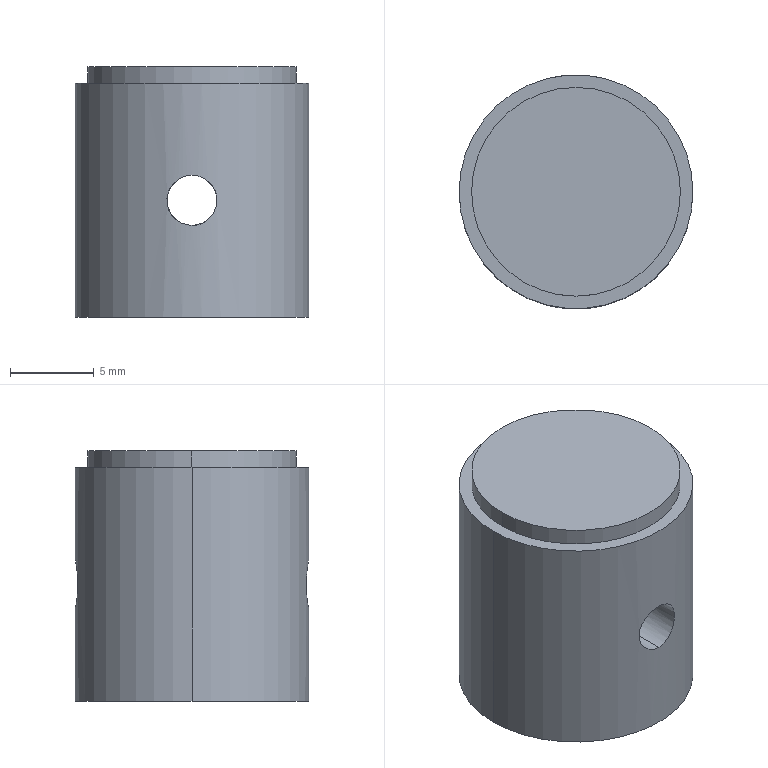Part | SolidWorks | features ICE 3, 3DProfileFeature 1, Extrusion 1, HoleWzd 1 | 1 solid | 17 faces | box 14 x 14 x 15 mm | volume 1304 mm3 | cylinder 10 | cone 4 | plane 3 | commonest cylinder face diameters 3 x4 9.5 x2 12.5 x2 14 x2
STEP:
#1=CARTESIAN_POINT('',(0.,-7.,5.5));
#2=VERTEX_POINT('',#1);
#3=CARTESIAN_POINT('',(0.,-7.,8.5));
#4=VERTEX_POINT('',#3);
#5=CARTESIAN_POINT('',(0.,-7.,5.5));
#6=CARTESIAN_POINT('',(-0.1961,-7.,5.5));
#7=CARTESIAN_POINT('',(-0.394,-6.991,5.54));
#8=CARTESIAN_POINT('',(-0.7552,-6.962,5.689));
#9=CARTESIAN_POINT('',(-0.9218,-6.94,5.801));
#10=CARTESIAN_POINT('',(-1.129,-6.909,6.008));
#11=CARTESIAN_POINT('',(-1.192,-6.898,6.085));
#12=CARTESIAN_POINT('',(-1.301,-6.878,6.247));
#13=CARTESIAN_POINT('',(-1.347,-6.869,6.333));
#14=CARTESIAN_POINT('',(-1.461,-6.846,6.606));
#15=CARTESIAN_POINT('',(-1.5,-6.837,6.801));
#16=CARTESIAN_POINT('',(-1.5,-6.837,7.098));
#17=CARTESIAN_POINT('',(-1.49,-6.84,7.196));
#18=CARTESIAN_POINT('',(-1.452,-6.848,7.388));
#19=CARTESIAN_POINT('',(-1.423,-6.854,7.484));
#20=CARTESIAN_POINT('',(-1.311,-6.877,7.756));
#21=CARTESIAN_POINT('',(-1.199,-6.898,7.922));
#22=CARTESIAN_POINT('',(-0.9236,-6.94,8.198));
#23=CARTESIAN_POINT('',(-0.7569,-6.961,8.31));
#24=CARTESIAN_POINT('',(-0.396,-6.991,8.46));
#25=CARTESIAN_POINT('',(-0.1988,-7.,8.5));
#26=CARTESIAN_POINT('',(0.,-7.,8.5));
#27=B_SPLINE_CURVE_WITH_KNOTS('',3,(#5,#6,#7,#8,#9,#10,#11,#12,#13,#14,#15,#16,#17,#18,#19,#20,#21,#22,#23,#24,#25,#26),.UNSPECIFIED.,.F.,.F.,(4,2,2,2,2,2,2,2,2,2,4),(0.004703,0.005291,0.005879,0.006173,0.006467,0.007054,0.007348,0.007642,0.00823,0.008818,0.009405),.UNSPECIFIED.);
#28=EDGE_CURVE('',#2,#4,#27,.T.);
#29=ORIENTED_EDGE('',*,*,#28,.F.);
#30=CARTESIAN_POINT('',(0.,-4.75,5.5));
#31=VERTEX_POINT('',#30);
#32=CARTESIAN_POINT('',(0.,-10.,5.5));
#33=DIRECTION('',(0.,1.,0.));
#34=VECTOR('',#33,1000.);
#35=LINE('',#32,#34);
#36=EDGE_CURVE('',#2,#31,#35,.T.);
#37=ORIENTED_EDGE('',*,*,#36,.T.);
#38=CARTESIAN_POINT('',(0.,-4.75,8.5));
#39=VERTEX_POINT('',#38);
#40=CARTESIAN_POINT('',(0.,-4.75,8.5));
#41=CARTESIAN_POINT('',(-0.0998,-4.75,8.5));
#42=CARTESIAN_POINT('',(-0.1978,-4.747,8.49));
#43=CARTESIAN_POINT('',(-0.3904,-4.735,8.452));
#44=CARTESIAN_POINT('',(-0.4861,-4.726,8.422));
#45=CARTESIAN_POINT('',(-0.6675,-4.704,8.347));
#46=CARTESIAN_POINT('',(-0.7534,-4.691,8.301));
#47=CARTESIAN_POINT('',(-0.916,-4.662,8.192));
#48=CARTESIAN_POINT('',(-0.9924,-4.646,8.129));
#49=CARTESIAN_POINT('',(-1.198,-4.598,7.923));
#50=CARTESIAN_POINT('',(-1.31,-4.566,7.757));
#51=CARTESIAN_POINT('',(-1.46,-4.521,7.396));
#52=CARTESIAN_POINT('',(-1.5,-4.507,7.198));
#53=CARTESIAN_POINT('',(-1.5,-4.507,6.902));
#54=CARTESIAN_POINT('',(-1.49,-4.51,6.802));
#55=CARTESIAN_POINT('',(-1.452,-4.523,6.609));
#56=CARTESIAN_POINT('',(-1.423,-4.532,6.515));
#57=CARTESIAN_POINT('',(-1.309,-4.567,6.242));
#58=CARTESIAN_POINT('',(-1.199,-4.598,6.077));
#59=CARTESIAN_POINT('',(-0.9911,-4.646,5.87));
#60=CARTESIAN_POINT('',(-0.9161,-4.662,5.808));
#61=CARTESIAN_POINT('',(-0.754,-4.691,5.7));
#62=CARTESIAN_POINT('',(-0.6661,-4.704,5.652));
#63=CARTESIAN_POINT('',(-0.395,-4.737,5.54));
#64=CARTESIAN_POINT('',(-0.1966,-4.75,5.5));
#65=CARTESIAN_POINT('',(0.,-4.75,5.5));
#66=B_SPLINE_CURVE_WITH_KNOTS('',3,(#40,#41,#42,#43,#44,#45,#46,#47,#48,#49,#50,#51,#52,#53,#54,#55,#56,#57,#58,#59,#60,#61,#62,#63,#64,#65),.UNSPECIFIED.,.F.,.F.,(4,2,2,2,2,2,2,2,2,2,2,2,4),(0.,0.000295,0.00059,0.000885,0.00118,0.00177,0.00236,0.002655,0.00295,0.00354,0.003835,0.00413,0.00472),.UNSPECIFIED.);
#67=EDGE_CURVE('',#39,#31,#66,.T.);
#68=ORIENTED_EDGE('',*,*,#67,.F.);
#69=CARTESIAN_POINT('',(0.,-10.,8.5));
#70=DIRECTION('',(0.,1.,0.));
#71=VECTOR('',#70,1000.);
#72=LINE('',#69,#71);
#73=EDGE_CURVE('',#4,#39,#72,.T.);
#74=ORIENTED_EDGE('',*,*,#73,.F.);
#75=EDGE_LOOP('',(#29,#37,#68,#74));
#76=FACE_OUTER_BOUND('',#75,.T.);
#77=CARTESIAN_POINT('',(0.,-10.,7.));
#78=DIRECTION('',(0.,1.,0.));
#79=DIRECTION('',(0.,0.,1.));
#80=AXIS2_PLACEMENT_3D('',#77,#78,#79);
#81=CYLINDRICAL_SURFACE('',#80,1.5);
#82=ADVANCED_FACE('',(#76),#81,.F.);
#83=CARTESIAN_POINT('',(0.,4.75,5.5));
#84=VERTEX_POINT('',#83);
#85=CARTESIAN_POINT('',(0.,4.75,8.5));
#86=VERTEX_POINT('',#85);
#87=CARTESIAN_POINT('',(0.,4.75,5.5));
#88=CARTESIAN_POINT('',(-0.1966,4.75,5.5));
#89=CARTESIAN_POINT('',(-0.3951,4.737,5.54));
#90=CARTESIAN_POINT('',(-0.6664,4.704,5.653));
#91=CARTESIAN_POINT('',(-0.7542,4.69,5.7));
#92=CARTESIAN_POINT('',(-0.9163,4.662,5.808));
#93=CARTESIAN_POINT('',(-0.9914,4.646,5.87));
#94=CARTESIAN_POINT('',(-1.199,4.598,6.078));
#95=CARTESIAN_POINT('',(-1.309,4.567,6.241));
#96=CARTESIAN_POINT('',(-1.423,4.532,6.515));
#97=CARTESIAN_POINT('',(-1.451,4.523,6.609));
#98=CARTESIAN_POINT('',(-1.49,4.51,6.801));
#99=CARTESIAN_POINT('',(-1.5,4.507,6.901));
#100=CARTESIAN_POINT('',(-1.5,4.507,7.099));
#101=CARTESIAN_POINT('',(-1.49,4.51,7.197));
#102=CARTESIAN_POINT('',(-1.452,4.523,7.39));
#103=CARTESIAN_POINT('',(-1.423,4.532,7.486));
#104=CARTESIAN_POINT('',(-1.31,4.567,7.757));
#105=CARTESIAN_POINT('',(-1.198,4.598,7.923));
#106=CARTESIAN_POINT('',(-0.9923,4.646,8.129));
#107=CARTESIAN_POINT('',(-0.9157,4.662,8.192));
#108=CARTESIAN_POINT('',(-0.7533,4.691,8.301));
#109=CARTESIAN_POINT('',(-0.6675,4.704,8.347));
#110=CARTESIAN_POINT('',(-0.4864,4.726,8.422));
#111=CARTESIAN_POINT('',(-0.3907,4.735,8.452));
#112=CARTESIAN_POINT('',(-0.1979,4.747,8.49));
#113=CARTESIAN_POINT('',(-0.09977,4.75,8.5));
#114=CARTESIAN_POINT('',(0.,4.75,8.5));
#115=B_SPLINE_CURVE_WITH_KNOTS('',3,(#87,#88,#89,#90,#91,#92,#93,#94,#95,#96,#97,#98,#99,#100,#101,#102,#103,#104,#105,#106,#107,#108,#109,#110,#111,#112,#113,#114),.UNSPECIFIED.,.F.,.F.,(4,2,2,2,2,2,2,2,2,2,2,2,2,4),(0.00472,0.00531,0.005605,0.0059,0.00649,0.006785,0.00708,0.007374,0.007669,0.008259,0.008554,0.008849,0.009144,0.009439),.UNSPECIFIED.);
#116=EDGE_CURVE('',#84,#86,#115,.T.);
#117=ORIENTED_EDGE('',*,*,#116,.F.);
#118=CARTESIAN_POINT('',(0.,7.,5.5));
#119=VERTEX_POINT('',#118);
#120=CARTESIAN_POINT('',(0.,-10.,5.5));
#121=DIRECTION('',(0.,1.,0.));
#122=VECTOR('',#121,1000.);
#123=LINE('',#120,#122);
#124=EDGE_CURVE('',#84,#119,#123,.T.);
#125=ORIENTED_EDGE('',*,*,#124,.T.);
#126=CARTESIAN_POINT('',(0.,7.,8.5));
#127=VERTEX_POINT('',#126);
#128=CARTESIAN_POINT('',(0.,7.,8.5));
#129=CARTESIAN_POINT('',(-0.09942,7.,8.5));
#130=CARTESIAN_POINT('',(-0.1971,6.998,8.49));
#131=CARTESIAN_POINT('',(-0.3892,6.99,8.452));
#132=CARTESIAN_POINT('',(-0.4847,6.984,8.423));
#133=CARTESIAN_POINT('',(-0.6662,6.969,8.348));
#134=CARTESIAN_POINT('',(-0.7523,6.96,8.301));
#135=CARTESIAN_POINT('',(-0.9151,6.94,8.193));
#136=CARTESIAN_POINT('',(-0.992,6.93,8.129));
#137=CARTESIAN_POINT('',(-1.199,6.898,7.922));
#138=CARTESIAN_POINT('',(-1.31,6.877,7.755));
#139=CARTESIAN_POINT('',(-1.46,6.846,7.395));
#140=CARTESIAN_POINT('',(-1.5,6.837,7.197));
#141=CARTESIAN_POINT('',(-1.5,6.837,6.902));
#142=CARTESIAN_POINT('',(-1.49,6.84,6.803));
#143=CARTESIAN_POINT('',(-1.452,6.848,6.61));
#144=CARTESIAN_POINT('',(-1.423,6.854,6.516));
#145=CARTESIAN_POINT('',(-1.31,6.877,6.243));
#146=CARTESIAN_POINT('',(-1.2,6.898,6.078));
#147=CARTESIAN_POINT('',(-0.9909,6.93,5.87));
#148=CARTESIAN_POINT('',(-0.9154,6.94,5.808));
#149=CARTESIAN_POINT('',(-0.7532,6.96,5.699));
#150=CARTESIAN_POINT('',(-0.6653,6.969,5.652));
#151=CARTESIAN_POINT('',(-0.4841,6.984,5.577));
#152=CARTESIAN_POINT('',(-0.3905,6.99,5.548));
#153=CARTESIAN_POINT('',(-0.1976,6.998,5.51));
#154=CARTESIAN_POINT('',(-0.09806,7.,5.5));
#155=CARTESIAN_POINT('',(0.,7.,5.5));
#156=B_SPLINE_CURVE_WITH_KNOTS('',3,(#128,#129,#130,#131,#132,#133,#134,#135,#136,#137,#138,#139,#140,#141,#142,#143,#144,#145,#146,#147,#148,#149,#150,#151,#152,#153,#154,#155),.UNSPECIFIED.,.F.,.F.,(4,2,2,2,2,2,2,2,2,2,2,2,2,4),(0.,0.000294,0.0005879,0.0008819,0.001176,0.001764,0.002352,0.002646,0.00294,0.003528,0.003821,0.004115,0.004409,0.004703),.UNSPECIFIED.);
#157=EDGE_CURVE('',#127,#119,#156,.T.);
#158=ORIENTED_EDGE('',*,*,#157,.F.);
#159=CARTESIAN_POINT('',(0.,-10.,8.5));
#160=DIRECTION('',(0.,1.,0.));
#161=VECTOR('',#160,1000.);
#162=LINE('',#159,#161);
#163=EDGE_CURVE('',#86,#127,#162,.T.);
#164=ORIENTED_EDGE('',*,*,#163,.F.);
#165=EDGE_LOOP('',(#117,#125,#158,#164));
#166=FACE_OUTER_BOUND('',#165,.T.);
#167=CARTESIAN_POINT('',(0.,-10.,7.));
#168=DIRECTION('',(0.,1.,0.));
#169=DIRECTION('',(0.,0.,1.));
#170=AXIS2_PLACEMENT_3D('',#167,#168,#169);
#171=CYLINDRICAL_SURFACE('',#170,1.5);
#172=ADVANCED_FACE('',(#166),#171,.F.);
#173=ORIENTED_EDGE('',*,*,#67,.T.);
#174=CARTESIAN_POINT('',(0.,-4.75,5.5));
#175=CARTESIAN_POINT('',(0.1966,-4.75,5.5));
#176=CARTESIAN_POINT('',(0.3951,-4.737,5.54));
#177=CARTESIAN_POINT('',(0.6664,-4.704,5.653));
#178=CARTESIAN_POINT('',(0.7542,-4.69,5.7));
#179=CARTESIAN_POINT('',(0.9163,-4.662,5.808));
#180=CARTESIAN_POINT('',(0.9914,-4.646,5.87));
#181=CARTESIAN_POINT('',(1.199,-4.598,6.078));
#182=CARTESIAN_POINT('',(1.309,-4.567,6.241));
#183=CARTESIAN_POINT('',(1.423,-4.532,6.515));
#184=CARTESIAN_POINT('',(1.451,-4.523,6.609));
#185=CARTESIAN_POINT('',(1.49,-4.51,6.801));
#186=CARTESIAN_POINT('',(1.5,-4.507,6.901));
#187=CARTESIAN_POINT('',(1.5,-4.507,7.099));
#188=CARTESIAN_POINT('',(1.49,-4.51,7.197));
#189=CARTESIAN_POINT('',(1.452,-4.523,7.39));
#190=CARTESIAN_POINT('',(1.423,-4.532,7.486));
#191=CARTESIAN_POINT('',(1.31,-4.567,7.757));
#192=CARTESIAN_POINT('',(1.198,-4.598,7.923));
#193=CARTESIAN_POINT('',(0.9923,-4.646,8.129));
#194=CARTESIAN_POINT('',(0.9157,-4.662,8.192));
#195=CARTESIAN_POINT('',(0.7533,-4.691,8.301));
#196=CARTESIAN_POINT('',(0.6675,-4.704,8.347));
#197=CARTESIAN_POINT('',(0.4864,-4.726,8.422));
#198=CARTESIAN_POINT('',(0.3907,-4.735,8.452));
#199=CARTESIAN_POINT('',(0.1979,-4.747,8.49));
#200=CARTESIAN_POINT('',(0.09977,-4.75,8.5));
#201=CARTESIAN_POINT('',(0.,-4.75,8.5));
#202=B_SPLINE_CURVE_WITH_KNOTS('',3,(#174,#175,#176,#177,#178,#179,#180,#181,#182,#183,#184,#185,#186,#187,#188,#189,#190,#191,#192,#193,#194,#195,#196,#197,#198,#199,#200,#201),.UNSPECIFIED.,.F.,.F.,(4,2,2,2,2,2,2,2,2,2,2,2,2,4),(0.00472,0.00531,0.005605,0.0059,0.00649,0.006785,0.00708,0.007374,0.007669,0.008259,0.008554,0.008849,0.009144,0.009439),.UNSPECIFIED.);
#203=EDGE_CURVE('',#31,#39,#202,.T.);
#204=ORIENTED_EDGE('',*,*,#203,.T.);
#205=EDGE_LOOP('',(#173,#204));
#206=FACE_BOUND('',#205,.T.);
#207=CARTESIAN_POINT('',(4.75,0.,11.));
#208=VERTEX_POINT('',#207);
#209=CARTESIAN_POINT('',(-4.75,0.,11.));
#210=VERTEX_POINT('',#209);
#211=CARTESIAN_POINT('',(0.,0.,11.));
#212=DIRECTION('',(0.,0.,-1.));
#213=DIRECTION('',(-1.,0.,0.));
#214=AXIS2_PLACEMENT_3D('',#211,#212,#213);
#215=CIRCLE('',#214,4.75);
#216=EDGE_CURVE('',#208,#210,#215,.T.);
#217=ORIENTED_EDGE('',*,*,#216,.F.);
#218=CARTESIAN_POINT('',(4.75,0.,3.984));
#219=VERTEX_POINT('',#218);
#220=CARTESIAN_POINT('',(4.75,0.,0.));
#221=DIRECTION('',(0.,0.,-1.));
#222=VECTOR('',#221,1000.);
#223=LINE('',#220,#222);
#224=EDGE_CURVE('',#208,#219,#223,.T.);
#225=ORIENTED_EDGE('',*,*,#224,.T.);
#226=CARTESIAN_POINT('',(-4.75,0.,3.984));
#227=VERTEX_POINT('',#226);
#228=CARTESIAN_POINT('',(0.,0.,3.984));
#229=DIRECTION('',(0.,0.,-1.));
#230=DIRECTION('',(-1.,0.,0.));
#231=AXIS2_PLACEMENT_3D('',#228,#229,#230);
#232=CIRCLE('',#231,4.75);
#233=EDGE_CURVE('',#219,#227,#232,.T.);
#234=ORIENTED_EDGE('',*,*,#233,.T.);
#235=CARTESIAN_POINT('',(-4.75,0.,0.));
#236=DIRECTION('',(0.,0.,-1.));
#237=VECTOR('',#236,1000.);
#238=LINE('',#235,#237);
#239=EDGE_CURVE('',#210,#227,#238,.T.);
#240=ORIENTED_EDGE('',*,*,#239,.F.);
#241=EDGE_LOOP('',(#217,#225,#234,#240));
#242=FACE_OUTER_BOUND('',#241,.T.);
#243=CARTESIAN_POINT('',(0.,0.,0.));
#244=DIRECTION('',(0.,0.,-1.));
#245=DIRECTION('',(-1.,0.,0.));
#246=AXIS2_PLACEMENT_3D('',#243,#244,#245);
#247=CYLINDRICAL_SURFACE('',#246,4.75);
#248=ADVANCED_FACE('',(#206,#242),#247,.F.);
#249=CARTESIAN_POINT('',(0.,0.,13.854));
#250=VERTEX_POINT('',#249);
#251=CARTESIAN_POINT('',(-4.75,0.,11.));
#252=DIRECTION('',(-0.8572,0.,-0.515));
#253=VECTOR('',#252,1000.);
#254=LINE('',#251,#253);
#255=EDGE_CURVE('',#250,#210,#254,.T.);
#256=ORIENTED_EDGE('',*,*,#255,.F.);
#257=CARTESIAN_POINT('',(4.75,0.,11.));
#258=DIRECTION('',(0.8572,0.,-0.515));
#259=VECTOR('',#258,1000.);
#260=LINE('',#257,#259);
#261=EDGE_CURVE('',#250,#208,#260,.T.);
#262=ORIENTED_EDGE('',*,*,#261,.T.);
#263=ORIENTED_EDGE('',*,*,#216,.T.);
#264=EDGE_LOOP('',(#256,#262,#263));
#265=FACE_OUTER_BOUND('',#264,.T.);
#266=CARTESIAN_POINT('',(0.,0.,11.));
#267=DIRECTION('',(0.,0.,-1.));
#268=DIRECTION('',(-1.,0.,0.));
#269=AXIS2_PLACEMENT_3D('',#266,#267,#268);
#270=CONICAL_SURFACE('',#269,4.75,1.03);
#271=ADVANCED_FACE('',(#265),#270,.F.);
#272=ORIENTED_EDGE('',*,*,#233,.F.);
#273=CARTESIAN_POINT('',(6.2,0.,0.));
#274=VERTEX_POINT('',#273);
#275=CARTESIAN_POINT('',(6.2,0.,0.));
#276=DIRECTION('',(0.342,0.,-0.9397));
#277=VECTOR('',#276,1000.);
#278=LINE('',#275,#277);
#279=EDGE_CURVE('',#219,#274,#278,.T.);
#280=ORIENTED_EDGE('',*,*,#279,.T.);
#281=CARTESIAN_POINT('',(-6.2,0.,0.));
#282=VERTEX_POINT('',#281);
#283=CARTESIAN_POINT('',(0.,0.,0.));
#284=DIRECTION('',(0.,0.,-1.));
#285=DIRECTION('',(-1.,0.,0.));
#286=AXIS2_PLACEMENT_3D('',#283,#284,#285);
#287=CIRCLE('',#286,6.2);
#288=EDGE_CURVE('',#274,#282,#287,.T.);
#289=ORIENTED_EDGE('',*,*,#288,.T.);
#290=CARTESIAN_POINT('',(-6.2,0.,0.));
#291=DIRECTION('',(-0.342,0.,-0.9397));
#292=VECTOR('',#291,1000.);
#293=LINE('',#290,#292);
#294=EDGE_CURVE('',#227,#282,#293,.T.);
#295=ORIENTED_EDGE('',*,*,#294,.F.);
#296=EDGE_LOOP('',(#272,#280,#289,#295));
#297=FACE_OUTER_BOUND('',#296,.T.);
#298=CARTESIAN_POINT('',(0.,0.,0.));
#299=DIRECTION('',(0.,0.,-1.));
#300=DIRECTION('',(-1.,0.,0.));
#301=AXIS2_PLACEMENT_3D('',#298,#299,#300);
#302=CONICAL_SURFACE('',#301,6.2,0.3491);
#303=ADVANCED_FACE('',(#297),#302,.F.);
#304=CARTESIAN_POINT('',(6.25,0.,14.));
#305=VERTEX_POINT('',#304);
#306=CARTESIAN_POINT('',(-6.25,0.,14.));
#307=VERTEX_POINT('',#306);
#308=CARTESIAN_POINT('',(0.,0.,14.));
#309=DIRECTION('',(0.,0.,1.));
#310=DIRECTION('',(1.,0.,0.));
#311=AXIS2_PLACEMENT_3D('',#308,#309,#310);
#312=CIRCLE('',#311,6.25);
#313=EDGE_CURVE('',#305,#307,#312,.T.);
#314=ORIENTED_EDGE('',*,*,#313,.T.);
#315=CARTESIAN_POINT('',(-6.25,0.,15.));
#316=VERTEX_POINT('',#315);
#317=CARTESIAN_POINT('',(-6.25,0.,14.));
#318=DIRECTION('',(0.,0.,1.));
#319=VECTOR('',#318,1000.);
#320=LINE('',#317,#319);
#321=EDGE_CURVE('',#307,#316,#320,.T.);
#322=ORIENTED_EDGE('',*,*,#321,.T.);
#323=CARTESIAN_POINT('',(6.25,0.,15.));
#324=VERTEX_POINT('',#323);
#325=CARTESIAN_POINT('',(0.,0.,15.));
#326=DIRECTION('',(0.,0.,1.));
#327=DIRECTION('',(1.,0.,0.));
#328=AXIS2_PLACEMENT_3D('',#325,#326,#327);
#329=CIRCLE('',#328,6.25);
#330=EDGE_CURVE('',#324,#316,#329,.T.);
#331=ORIENTED_EDGE('',*,*,#330,.F.);
#332=CARTESIAN_POINT('',(6.25,0.,14.));
#333=DIRECTION('',(0.,0.,1.));
#334=VECTOR('',#333,1000.);
#335=LINE('',#332,#334);
#336=EDGE_CURVE('',#305,#324,#335,.T.);
#337=ORIENTED_EDGE('',*,*,#336,.F.);
#338=EDGE_LOOP('',(#314,#322,#331,#337));
#339=FACE_OUTER_BOUND('',#338,.T.);
#340=CARTESIAN_POINT('',(0.,0.,14.));
#341=DIRECTION('',(0.,0.,1.));
#342=DIRECTION('',(1.,0.,0.));
#343=AXIS2_PLACEMENT_3D('',#340,#341,#342);
#344=CYLINDRICAL_SURFACE('',#343,6.25);
#345=ADVANCED_FACE('',(#339),#344,.T.);
#346=ORIENTED_EDGE('',*,*,#157,.T.);
#347=CARTESIAN_POINT('',(0.,7.,5.5));
#348=CARTESIAN_POINT('',(0.1961,7.,5.5));
#349=CARTESIAN_POINT('',(0.394,6.991,5.54));
#350=CARTESIAN_POINT('',(0.7552,6.962,5.689));
#351=CARTESIAN_POINT('',(0.9218,6.94,5.801));
#352=CARTESIAN_POINT('',(1.129,6.909,6.008));
#353=CARTESIAN_POINT('',(1.192,6.898,6.085));
#354=CARTESIAN_POINT('',(1.301,6.878,6.247));
#355=CARTESIAN_POINT('',(1.347,6.869,6.333));
#356=CARTESIAN_POINT('',(1.461,6.846,6.606));
#357=CARTESIAN_POINT('',(1.5,6.837,6.801));
#358=CARTESIAN_POINT('',(1.5,6.837,7.098));
#359=CARTESIAN_POINT('',(1.49,6.84,7.196));
#360=CARTESIAN_POINT('',(1.452,6.848,7.388));
#361=CARTESIAN_POINT('',(1.423,6.854,7.484));
#362=CARTESIAN_POINT('',(1.311,6.877,7.756));
#363=CARTESIAN_POINT('',(1.199,6.898,7.922));
#364=CARTESIAN_POINT('',(0.9236,6.94,8.198));
#365=CARTESIAN_POINT('',(0.7569,6.961,8.31));
#366=CARTESIAN_POINT('',(0.396,6.991,8.46));
#367=CARTESIAN_POINT('',(0.1988,7.,8.5));
#368=CARTESIAN_POINT('',(0.,7.,8.5));
#369=B_SPLINE_CURVE_WITH_KNOTS('',3,(#347,#348,#349,#350,#351,#352,#353,#354,#355,#356,#357,#358,#359,#360,#361,#362,#363,#364,#365,#366,#367,#368),.UNSPECIFIED.,.F.,.F.,(4,2,2,2,2,2,2,2,2,2,4),(0.004703,0.005291,0.005879,0.006173,0.006467,0.007054,0.007348,0.007642,0.00823,0.008818,0.009405),.UNSPECIFIED.);
#370=EDGE_CURVE('',#119,#127,#369,.T.);
#371=ORIENTED_EDGE('',*,*,#370,.T.);
#372=EDGE_LOOP('',(#346,#371));
#373=FACE_BOUND('',#372,.T.);
#374=CARTESIAN_POINT('',(7.,0.,14.));
#375=VERTEX_POINT('',#374);
#376=CARTESIAN_POINT('',(-7.,0.,14.));
#377=VERTEX_POINT('',#376);
#378=CARTESIAN_POINT('',(0.,0.,14.));
#379=DIRECTION('',(0.,0.,1.));
#380=DIRECTION('',(1.,0.,0.));
#381=AXIS2_PLACEMENT_3D('',#378,#379,#380);
#382=CIRCLE('',#381,7.);
#383=EDGE_CURVE('',#375,#377,#382,.T.);
#384=ORIENTED_EDGE('',*,*,#383,.F.);
#385=CARTESIAN_POINT('',(7.,0.,0.));
#386=VERTEX_POINT('',#385);
#387=CARTESIAN_POINT('',(7.,0.,15.));
#388=DIRECTION('',(0.,0.,-1.));
#389=VECTOR('',#388,1000.);
#390=LINE('',#387,#389);
#391=EDGE_CURVE('',#375,#386,#390,.T.);
#392=ORIENTED_EDGE('',*,*,#391,.T.);
#393=CARTESIAN_POINT('',(-7.,0.,0.));
#394=VERTEX_POINT('',#393);
#395=CARTESIAN_POINT('',(0.,0.,0.));
#396=DIRECTION('',(0.,0.,1.));
#397=DIRECTION('',(1.,0.,0.));
#398=AXIS2_PLACEMENT_3D('',#395,#396,#397);
#399=CIRCLE('',#398,7.);
#400=EDGE_CURVE('',#386,#394,#399,.T.);
#401=ORIENTED_EDGE('',*,*,#400,.T.);
#402=CARTESIAN_POINT('',(-7.,0.,15.));
#403=DIRECTION('',(0.,0.,-1.));
#404=VECTOR('',#403,1000.);
#405=LINE('',#402,#404);
#406=EDGE_CURVE('',#377,#394,#405,.T.);
#407=ORIENTED_EDGE('',*,*,#406,.F.);
#408=EDGE_LOOP('',(#384,#392,#401,#407));
#409=FACE_OUTER_BOUND('',#408,.T.);
#410=CARTESIAN_POINT('',(0.,0.,15.));
#411=DIRECTION('',(0.,0.,-1.));
#412=DIRECTION('',(-1.,0.,0.));
#413=AXIS2_PLACEMENT_3D('',#410,#411,#412);
#414=CYLINDRICAL_SURFACE('',#413,7.);
#415=ADVANCED_FACE('',(#373,#409),#414,.T.);
#416=ORIENTED_EDGE('',*,*,#391,.F.);
#417=CARTESIAN_POINT('',(0.,0.,14.));
#418=DIRECTION('',(0.,0.,1.));
#419=DIRECTION('',(1.,0.,0.));
#420=AXIS2_PLACEMENT_3D('',#417,#418,#419);
#421=CIRCLE('',#420,7.);
#422=EDGE_CURVE('',#377,#375,#421,.T.);
#423=ORIENTED_EDGE('',*,*,#422,.F.);
#424=ORIENTED_EDGE('',*,*,#406,.T.);
#425=CARTESIAN_POINT('',(0.,0.,0.));
#426=DIRECTION('',(0.,0.,1.));
#427=DIRECTION('',(1.,0.,0.));
#428=AXIS2_PLACEMENT_3D('',#425,#426,#427);
#429=CIRCLE('',#428,7.);
#430=EDGE_CURVE('',#394,#386,#429,.T.);
#431=ORIENTED_EDGE('',*,*,#430,.T.);
#432=EDGE_LOOP('',(#416,#423,#424,#431));
#433=FACE_OUTER_BOUND('',#432,.T.);
#434=CARTESIAN_POINT('',(0.,-7.,8.5));
#435=CARTESIAN_POINT('',(0.09942,-7.,8.5));
#436=CARTESIAN_POINT('',(0.1971,-6.998,8.49));
#437=CARTESIAN_POINT('',(0.3892,-6.99,8.452));
#438=CARTESIAN_POINT('',(0.4847,-6.984,8.423));
#439=CARTESIAN_POINT('',(0.6662,-6.969,8.348));
#440=CARTESIAN_POINT('',(0.7523,-6.96,8.301));
#441=CARTESIAN_POINT('',(0.9151,-6.94,8.193));
#442=CARTESIAN_POINT('',(0.992,-6.93,8.129));
#443=CARTESIAN_POINT('',(1.199,-6.898,7.922));
#444=CARTESIAN_POINT('',(1.31,-6.877,7.755));
#445=CARTESIAN_POINT('',(1.46,-6.846,7.395));
#446=CARTESIAN_POINT('',(1.5,-6.837,7.197));
#447=CARTESIAN_POINT('',(1.5,-6.837,6.902));
#448=CARTESIAN_POINT('',(1.49,-6.84,6.803));
#449=CARTESIAN_POINT('',(1.452,-6.848,6.61));
#450=CARTESIAN_POINT('',(1.423,-6.854,6.516));
#451=CARTESIAN_POINT('',(1.31,-6.877,6.243));
#452=CARTESIAN_POINT('',(1.2,-6.898,6.078));
#453=CARTESIAN_POINT('',(0.9909,-6.93,5.87));
#454=CARTESIAN_POINT('',(0.9154,-6.94,5.808));
#455=CARTESIAN_POINT('',(0.7532,-6.96,5.699));
#456=CARTESIAN_POINT('',(0.6653,-6.969,5.652));
#457=CARTESIAN_POINT('',(0.4841,-6.984,5.577));
#458=CARTESIAN_POINT('',(0.3905,-6.99,5.548));
#459=CARTESIAN_POINT('',(0.1976,-6.998,5.51));
#460=CARTESIAN_POINT('',(0.09806,-7.,5.5));
#461=CARTESIAN_POINT('',(0.,-7.,5.5));
#462=B_SPLINE_CURVE_WITH_KNOTS('',3,(#434,#435,#436,#437,#438,#439,#440,#441,#442,#443,#444,#445,#446,#447,#448,#449,#450,#451,#452,#453,#454,#455,#456,#457,#458,#459,#460,#461),.UNSPECIFIED.,.F.,.F.,(4,2,2,2,2,2,2,2,2,2,2,2,2,4),(0.,0.000294,0.0005879,0.0008819,0.001176,0.001764,0.002352,0.002646,0.00294,0.003528,0.003821,0.004115,0.004409,0.004703),.UNSPECIFIED.);
#463=EDGE_CURVE('',#4,#2,#462,.T.);
#464=ORIENTED_EDGE('',*,*,#463,.T.);
#465=ORIENTED_EDGE('',*,*,#28,.T.);
#466=EDGE_LOOP('',(#464,#465));
#467=FACE_BOUND('',#466,.T.);
#468=CARTESIAN_POINT('',(0.,0.,15.));
#469=DIRECTION('',(0.,0.,-1.));
#470=DIRECTION('',(-1.,0.,0.));
#471=AXIS2_PLACEMENT_3D('',#468,#469,#470);
#472=CYLINDRICAL_SURFACE('',#471,7.);
#473=ADVANCED_FACE('',(#433,#467),#472,.T.);
#474=CARTESIAN_POINT('',(0.,0.,0.));
#475=DIRECTION('',(0.,0.,-1.));
#476=DIRECTION('',(-1.,0.,0.));
#477=AXIS2_PLACEMENT_3D('',#474,#475,#476);
#478=CIRCLE('',#477,6.2);
#479=EDGE_CURVE('',#282,#274,#478,.T.);
#480=ORIENTED_EDGE('',*,*,#479,.F.);
#481=ORIENTED_EDGE('',*,*,#288,.F.);
#482=EDGE_LOOP('',(#480,#481));
#483=FACE_BOUND('',#482,.T.);
#484=ORIENTED_EDGE('',*,*,#430,.F.);
#485=ORIENTED_EDGE('',*,*,#400,.F.);
#486=EDGE_LOOP('',(#484,#485));
#487=FACE_OUTER_BOUND('',#486,.T.);
#488=CARTESIAN_POINT('',(0.,0.,0.));
#489=DIRECTION('',(0.,0.,1.));
#490=DIRECTION('',(1.,0.,0.));
#491=AXIS2_PLACEMENT_3D('',#488,#489,#490);
#492=PLANE('',#491);
#493=ADVANCED_FACE('',(#483,#487),#492,.F.);
#494=ORIENTED_EDGE('',*,*,#313,.F.);
#495=CARTESIAN_POINT('',(0.,0.,14.));
#496=DIRECTION('',(0.,0.,1.));
#497=DIRECTION('',(1.,0.,0.));
#498=AXIS2_PLACEMENT_3D('',#495,#496,#497);
#499=CIRCLE('',#498,6.25);
#500=EDGE_CURVE('',#307,#305,#499,.T.);
#501=ORIENTED_EDGE('',*,*,#500,.F.);
#502=EDGE_LOOP('',(#494,#501));
#503=FACE_BOUND('',#502,.T.);
#504=ORIENTED_EDGE('',*,*,#422,.T.);
#505=ORIENTED_EDGE('',*,*,#383,.T.);
#506=EDGE_LOOP('',(#504,#505));
#507=FACE_OUTER_BOUND('',#506,.T.);
#508=CARTESIAN_POINT('',(0.,0.,14.));
#509=DIRECTION('',(0.,0.,1.));
#510=DIRECTION('',(1.,0.,0.));
#511=AXIS2_PLACEMENT_3D('',#508,#509,#510);
#512=PLANE('',#511);
#513=ADVANCED_FACE('',(#503,#507),#512,.T.);
#514=ORIENTED_EDGE('',*,*,#321,.F.);
#515=ORIENTED_EDGE('',*,*,#500,.T.);
#516=ORIENTED_EDGE('',*,*,#336,.T.);
#517=CARTESIAN_POINT('',(0.,0.,15.));
#518=DIRECTION('',(0.,0.,1.));
#519=DIRECTION('',(1.,0.,0.));
#520=AXIS2_PLACEMENT_3D('',#517,#518,#519);
#521=CIRCLE('',#520,6.25);
#522=EDGE_CURVE('',#316,#324,#521,.T.);
#523=ORIENTED_EDGE('',*,*,#522,.F.);
#524=EDGE_LOOP('',(#514,#515,#516,#523));
#525=FACE_OUTER_BOUND('',#524,.T.);
#526=CARTESIAN_POINT('',(0.,0.,14.));
#527=DIRECTION('',(0.,0.,1.));
#528=DIRECTION('',(1.,0.,0.));
#529=AXIS2_PLACEMENT_3D('',#526,#527,#528);
#530=CYLINDRICAL_SURFACE('',#529,6.25);
#531=ADVANCED_FACE('',(#525),#530,.T.);
#532=ORIENTED_EDGE('',*,*,#330,.T.);
#533=ORIENTED_EDGE('',*,*,#522,.T.);
#534=EDGE_LOOP('',(#532,#533));
#535=FACE_OUTER_BOUND('',#534,.T.);
#536=CARTESIAN_POINT('',(0.,0.,15.));
#537=DIRECTION('',(0.,0.,1.));
#538=DIRECTION('',(1.,0.,0.));
#539=AXIS2_PLACEMENT_3D('',#536,#537,#538);
#540=PLANE('',#539);
#541=ADVANCED_FACE('',(#535),#540,.T.);
#542=ORIENTED_EDGE('',*,*,#279,.F.);
#543=CARTESIAN_POINT('',(0.,0.,3.984));
#544=DIRECTION('',(0.,0.,-1.));
#545=DIRECTION('',(-1.,0.,0.));
#546=AXIS2_PLACEMENT_3D('',#543,#544,#545);
#547=CIRCLE('',#546,4.75);
#548=EDGE_CURVE('',#227,#219,#547,.T.);
#549=ORIENTED_EDGE('',*,*,#548,.F.);
#550=ORIENTED_EDGE('',*,*,#294,.T.);
#551=ORIENTED_EDGE('',*,*,#479,.T.);
#552=EDGE_LOOP('',(#542,#549,#550,#551));
#553=FACE_OUTER_BOUND('',#552,.T.);
#554=CARTESIAN_POINT('',(0.,0.,0.));
#555=DIRECTION('',(0.,0.,-1.));
#556=DIRECTION('',(-1.,0.,0.));
#557=AXIS2_PLACEMENT_3D('',#554,#555,#556);
#558=CONICAL_SURFACE('',#557,6.2,0.3491);
#559=ADVANCED_FACE('',(#553),#558,.F.);
#560=ORIENTED_EDGE('',*,*,#261,.F.);
#561=ORIENTED_EDGE('',*,*,#255,.T.);
#562=CARTESIAN_POINT('',(0.,0.,11.));
#563=DIRECTION('',(0.,0.,-1.));
#564=DIRECTION('',(-1.,0.,0.));
#565=AXIS2_PLACEMENT_3D('',#562,#563,#564);
#566=CIRCLE('',#565,4.75);
#567=EDGE_CURVE('',#210,#208,#566,.T.);
#568=ORIENTED_EDGE('',*,*,#567,.T.);
#569=EDGE_LOOP('',(#560,#561,#568));
#570=FACE_OUTER_BOUND('',#569,.T.);
#571=CARTESIAN_POINT('',(0.,0.,11.));
#572=DIRECTION('',(0.,0.,-1.));
#573=DIRECTION('',(-1.,0.,0.));
#574=AXIS2_PLACEMENT_3D('',#571,#572,#573);
#575=CONICAL_SURFACE('',#574,4.75,1.03);
#576=ADVANCED_FACE('',(#570),#575,.F.);
#577=ORIENTED_EDGE('',*,*,#224,.F.);
#578=ORIENTED_EDGE('',*,*,#567,.F.);
#579=ORIENTED_EDGE('',*,*,#239,.T.);
#580=ORIENTED_EDGE('',*,*,#548,.T.);
#581=EDGE_LOOP('',(#577,#578,#579,#580));
#582=FACE_OUTER_BOUND('',#581,.T.);
#583=CARTESIAN_POINT('',(0.,4.75,8.5));
#584=CARTESIAN_POINT('',(0.0998,4.75,8.5));
#585=CARTESIAN_POINT('',(0.1978,4.747,8.49));
#586=CARTESIAN_POINT('',(0.3904,4.735,8.452));
#587=CARTESIAN_POINT('',(0.4861,4.726,8.422));
#588=CARTESIAN_POINT('',(0.6675,4.704,8.347));
#589=CARTESIAN_POINT('',(0.7534,4.691,8.301));
#590=CARTESIAN_POINT('',(0.916,4.662,8.192));
#591=CARTESIAN_POINT('',(0.9924,4.646,8.129));
#592=CARTESIAN_POINT('',(1.198,4.598,7.923));
#593=CARTESIAN_POINT('',(1.31,4.566,7.757));
#594=CARTESIAN_POINT('',(1.46,4.521,7.396));
#595=CARTESIAN_POINT('',(1.5,4.507,7.198));
#596=CARTESIAN_POINT('',(1.5,4.507,6.902));
#597=CARTESIAN_POINT('',(1.49,4.51,6.802));
#598=CARTESIAN_POINT('',(1.452,4.523,6.609));
#599=CARTESIAN_POINT('',(1.423,4.532,6.515));
#600=CARTESIAN_POINT('',(1.309,4.567,6.242));
#601=CARTESIAN_POINT('',(1.199,4.598,6.077));
#602=CARTESIAN_POINT('',(0.9911,4.646,5.87));
#603=CARTESIAN_POINT('',(0.9161,4.662,5.808));
#604=CARTESIAN_POINT('',(0.754,4.691,5.7));
#605=CARTESIAN_POINT('',(0.6661,4.704,5.652));
#606=CARTESIAN_POINT('',(0.395,4.737,5.54));
#607=CARTESIAN_POINT('',(0.1966,4.75,5.5));
#608=CARTESIAN_POINT('',(0.,4.75,5.5));
#609=B_SPLINE_CURVE_WITH_KNOTS('',3,(#583,#584,#585,#586,#587,#588,#589,#590,#591,#592,#593,#594,#595,#596,#597,#598,#599,#600,#601,#602,#603,#604,#605,#606,#607,#608),.UNSPECIFIED.,.F.,.F.,(4,2,2,2,2,2,2,2,2,2,2,2,4),(0.,0.000295,0.00059,0.000885,0.00118,0.00177,0.00236,0.002655,0.00295,0.00354,0.003835,0.00413,0.00472),.UNSPECIFIED.);
#610=EDGE_CURVE('',#86,#84,#609,.T.);
#611=ORIENTED_EDGE('',*,*,#610,.T.);
#612=ORIENTED_EDGE('',*,*,#116,.T.);
#613=EDGE_LOOP('',(#611,#612));
#614=FACE_BOUND('',#613,.T.);
#615=CARTESIAN_POINT('',(0.,0.,0.));
#616=DIRECTION('',(0.,0.,-1.));
#617=DIRECTION('',(-1.,0.,0.));
#618=AXIS2_PLACEMENT_3D('',#615,#616,#617);
#619=CYLINDRICAL_SURFACE('',#618,4.75);
#620=ADVANCED_FACE('',(#582,#614),#619,.F.);
#621=ORIENTED_EDGE('',*,*,#124,.F.);
#622=ORIENTED_EDGE('',*,*,#610,.F.);
#623=ORIENTED_EDGE('',*,*,#163,.T.);
#624=ORIENTED_EDGE('',*,*,#370,.F.);
#625=EDGE_LOOP('',(#621,#622,#623,#624));
#626=FACE_OUTER_BOUND('',#625,.T.);
#627=CARTESIAN_POINT('',(0.,-10.,7.));
#628=DIRECTION('',(0.,1.,0.));
#629=DIRECTION('',(0.,0.,1.));
#630=AXIS2_PLACEMENT_3D('',#627,#628,#629);
#631=CYLINDRICAL_SURFACE('',#630,1.5);
#632=ADVANCED_FACE('',(#626),#631,.F.);
#633=ORIENTED_EDGE('',*,*,#36,.F.);
#634=ORIENTED_EDGE('',*,*,#463,.F.);
#635=ORIENTED_EDGE('',*,*,#73,.T.);
#636=ORIENTED_EDGE('',*,*,#203,.F.);
#637=EDGE_LOOP('',(#633,#634,#635,#636));
#638=FACE_OUTER_BOUND('',#637,.T.);
#639=CARTESIAN_POINT('',(0.,-10.,7.));
#640=DIRECTION('',(0.,1.,0.));
#641=DIRECTION('',(0.,0.,1.));
#642=AXIS2_PLACEMENT_3D('',#639,#640,#641);
#643=CYLINDRICAL_SURFACE('',#642,1.5);
#644=ADVANCED_FACE('',(#638),#643,.F.);
#645=CLOSED_SHELL('',(#82,#172,#248,#271,#303,#345,#415,#473,#493,#513,#531,#541,#559,#576,#620,#632,#644));
#646=MANIFOLD_SOLID_BREP('',#645);
#647=CARTESIAN_POINT('',(0.,0.,0.));
#648=DIRECTION('',(0.,0.,1.));
#649=DIRECTION('',(1.,0.,0.));
#650=AXIS2_PLACEMENT_3D('',#647,#648,#649);
#651=(LENGTH_UNIT()NAMED_UNIT(*)SI_UNIT(.MILLI.,.METRE.));
#652=UNCERTAINTY_MEASURE_WITH_UNIT(LENGTH_MEASURE(0.00001),#651,'','');
#653=(NAMED_UNIT(*)PLANE_ANGLE_UNIT()SI_UNIT($,.RADIAN.));
#654=(NAMED_UNIT(*)SI_UNIT($,.STERADIAN.)SOLID_ANGLE_UNIT());
#655=(GEOMETRIC_REPRESENTATION_CONTEXT(3)GLOBAL_UNCERTAINTY_ASSIGNED_CONTEXT((#652))GLOBAL_UNIT_ASSIGNED_CONTEXT((#651,#653,#654))REPRESENTATION_CONTEXT('',''));
#656=ADVANCED_BREP_SHAPE_REPRESENTATION('',(#646,#650),#655);